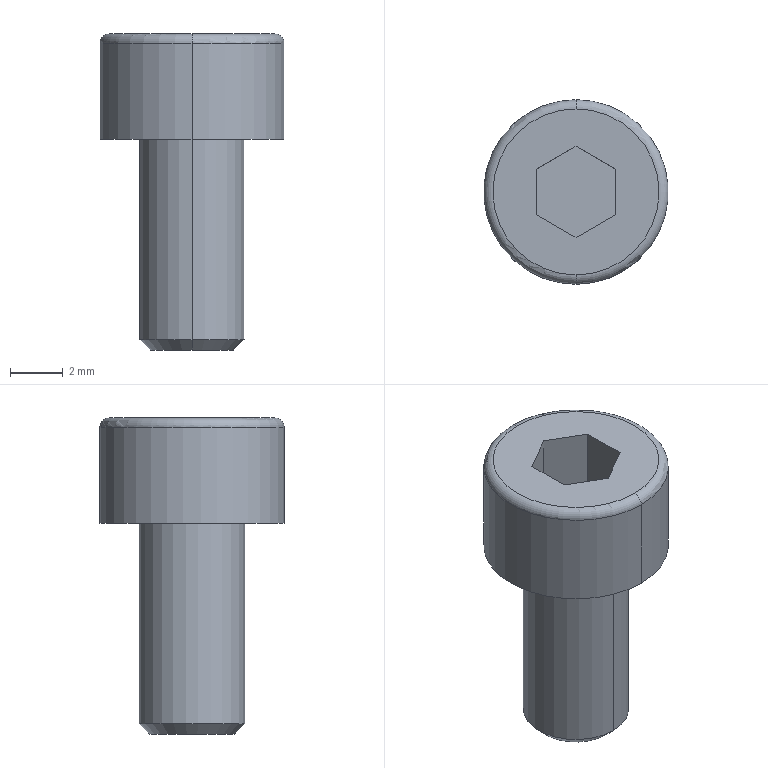Part | SolidWorks | features Chamfer 1, Fillet 1, ICE 1, Revolution 1 | 1 solid | 18 faces | box 7 x 7 x 12 mm | volume 233.87 mm3 | plane 10 | cylinder 4 | cone 2 | torus 2 | commonest cylinder face diameters 4 x2 7 x2
STEP:
#1=CARTESIAN_POINT('',(0.,1.6,-8.));
#2=VERTEX_POINT('',#1);
#3=CARTESIAN_POINT('',(0.,-1.6,-8.));
#4=VERTEX_POINT('',#3);
#5=CARTESIAN_POINT('',(0.,0.,-8.));
#6=DIRECTION('',(0.,0.,-1.));
#7=DIRECTION('',(0.,-1.,0.));
#8=AXIS2_PLACEMENT_3D('',#5,#6,#7);
#9=CIRCLE('',#8,1.6);
#10=EDGE_CURVE('',#2,#4,#9,.T.);
#11=ORIENTED_EDGE('',*,*,#10,.F.);
#12=CARTESIAN_POINT('',(0.,2.,-7.6));
#13=VERTEX_POINT('',#12);
#14=CARTESIAN_POINT('',(0.,2.,-7.6));
#15=DIRECTION('',(0.,0.7071,0.7071));
#16=VECTOR('',#15,1000.);
#17=LINE('',#14,#16);
#18=EDGE_CURVE('',#2,#13,#17,.T.);
#19=ORIENTED_EDGE('',*,*,#18,.T.);
#20=CARTESIAN_POINT('',(0.,-2.,-7.6));
#21=VERTEX_POINT('',#20);
#22=CARTESIAN_POINT('',(0.,0.,-7.6));
#23=DIRECTION('',(0.,0.,1.));
#24=DIRECTION('',(0.,-1.,0.));
#25=AXIS2_PLACEMENT_3D('',#22,#23,#24);
#26=CIRCLE('',#25,2.);
#27=EDGE_CURVE('',#21,#13,#26,.T.);
#28=ORIENTED_EDGE('',*,*,#27,.F.);
#29=CARTESIAN_POINT('',(0.,-2.,-7.6));
#30=DIRECTION('',(0.,-0.7071,0.7071));
#31=VECTOR('',#30,1000.);
#32=LINE('',#29,#31);
#33=EDGE_CURVE('',#4,#21,#32,.T.);
#34=ORIENTED_EDGE('',*,*,#33,.F.);
#35=EDGE_LOOP('',(#11,#19,#28,#34));
#36=FACE_OUTER_BOUND('',#35,.T.);
#37=CARTESIAN_POINT('',(0.,0.,-7.6));
#38=DIRECTION('',(0.,0.,1.));
#39=DIRECTION('',(0.,-1.,0.));
#40=AXIS2_PLACEMENT_3D('',#37,#38,#39);
#41=CONICAL_SURFACE('',#40,2.,0.7854);
#42=ADVANCED_FACE('',(#36),#41,.T.);
#43=CARTESIAN_POINT('',(0.,-3.15,4.));
#44=VERTEX_POINT('',#43);
#45=CARTESIAN_POINT('',(0.,3.15,4.));
#46=VERTEX_POINT('',#45);
#47=CARTESIAN_POINT('',(0.,0.,4.));
#48=DIRECTION('',(0.,0.,1.));
#49=DIRECTION('',(0.,1.,0.));
#50=AXIS2_PLACEMENT_3D('',#47,#48,#49);
#51=CIRCLE('',#50,3.15);
#52=EDGE_CURVE('',#44,#46,#51,.T.);
#53=ORIENTED_EDGE('',*,*,#52,.F.);
#54=CARTESIAN_POINT('',(0.,-3.5,3.65));
#55=VERTEX_POINT('',#54);
#56=CARTESIAN_POINT('',(0.,-3.15,3.65));
#57=DIRECTION('',(1.,0.,0.));
#58=DIRECTION('',(0.,1.,0.));
#59=AXIS2_PLACEMENT_3D('',#56,#57,#58);
#60=CIRCLE('',#59,0.35);
#61=EDGE_CURVE('',#44,#55,#60,.T.);
#62=ORIENTED_EDGE('',*,*,#61,.T.);
#63=CARTESIAN_POINT('',(0.,3.5,3.65));
#64=VERTEX_POINT('',#63);
#65=CARTESIAN_POINT('',(0.,0.,3.65));
#66=DIRECTION('',(0.,0.,-1.));
#67=DIRECTION('',(0.,1.,0.));
#68=AXIS2_PLACEMENT_3D('',#65,#66,#67);
#69=CIRCLE('',#68,3.5);
#70=EDGE_CURVE('',#64,#55,#69,.T.);
#71=ORIENTED_EDGE('',*,*,#70,.F.);
#72=CARTESIAN_POINT('',(0.,3.15,3.65));
#73=DIRECTION('',(-1.,0.,0.));
#74=DIRECTION('',(0.,0.,1.));
#75=AXIS2_PLACEMENT_3D('',#72,#73,#74);
#76=CIRCLE('',#75,0.35);
#77=EDGE_CURVE('',#46,#64,#76,.T.);
#78=ORIENTED_EDGE('',*,*,#77,.F.);
#79=EDGE_LOOP('',(#53,#62,#71,#78));
#80=FACE_OUTER_BOUND('',#79,.T.);
#81=CARTESIAN_POINT('',(0.,0.,3.65));
#82=DIRECTION('',(0.,0.,-1.));
#83=DIRECTION('',(0.,1.,0.));
#84=AXIS2_PLACEMENT_3D('',#81,#82,#83);
#85=TOROIDAL_SURFACE('',#84,3.15,0.35);
#86=ADVANCED_FACE('',(#80),#85,.T.);
#87=ORIENTED_EDGE('',*,*,#27,.T.);
#88=CARTESIAN_POINT('',(0.,2.,0.));
#89=VERTEX_POINT('',#88);
#90=CARTESIAN_POINT('',(0.,2.,4.));
#91=DIRECTION('',(0.,0.,1.));
#92=VECTOR('',#91,1000.);
#93=LINE('',#90,#92);
#94=EDGE_CURVE('',#13,#89,#93,.T.);
#95=ORIENTED_EDGE('',*,*,#94,.T.);
#96=CARTESIAN_POINT('',(0.,-2.,0.));
#97=VERTEX_POINT('',#96);
#98=CARTESIAN_POINT('',(0.,0.,0.));
#99=DIRECTION('',(0.,0.,1.));
#100=DIRECTION('',(0.,-1.,0.));
#101=AXIS2_PLACEMENT_3D('',#98,#99,#100);
#102=CIRCLE('',#101,2.);
#103=EDGE_CURVE('',#97,#89,#102,.T.);
#104=ORIENTED_EDGE('',*,*,#103,.F.);
#105=CARTESIAN_POINT('',(0.,-2.,4.));
#106=DIRECTION('',(0.,0.,1.));
#107=VECTOR('',#106,1000.);
#108=LINE('',#105,#107);
#109=EDGE_CURVE('',#21,#97,#108,.T.);
#110=ORIENTED_EDGE('',*,*,#109,.F.);
#111=EDGE_LOOP('',(#87,#95,#104,#110));
#112=FACE_OUTER_BOUND('',#111,.T.);
#113=CARTESIAN_POINT('',(0.,0.,4.));
#114=DIRECTION('',(0.,0.,1.));
#115=DIRECTION('',(0.,-1.,0.));
#116=AXIS2_PLACEMENT_3D('',#113,#114,#115);
#117=CYLINDRICAL_SURFACE('',#116,2.);
#118=ADVANCED_FACE('',(#112),#117,.T.);
#119=CARTESIAN_POINT('',(0.,-3.5,0.));
#120=VERTEX_POINT('',#119);
#121=CARTESIAN_POINT('',(0.,3.5,0.));
#122=VERTEX_POINT('',#121);
#123=CARTESIAN_POINT('',(0.,0.,0.));
#124=DIRECTION('',(0.,0.,1.));
#125=DIRECTION('',(0.,-1.,0.));
#126=AXIS2_PLACEMENT_3D('',#123,#124,#125);
#127=CIRCLE('',#126,3.5);
#128=EDGE_CURVE('',#120,#122,#127,.T.);
#129=ORIENTED_EDGE('',*,*,#128,.T.);
#130=CARTESIAN_POINT('',(0.,3.5,4.));
#131=DIRECTION('',(0.,0.,1.));
#132=VECTOR('',#131,1000.);
#133=LINE('',#130,#132);
#134=EDGE_CURVE('',#122,#64,#133,.T.);
#135=ORIENTED_EDGE('',*,*,#134,.T.);
#136=ORIENTED_EDGE('',*,*,#70,.T.);
#137=CARTESIAN_POINT('',(0.,-3.5,4.));
#138=DIRECTION('',(0.,0.,1.));
#139=VECTOR('',#138,1000.);
#140=LINE('',#137,#139);
#141=EDGE_CURVE('',#120,#55,#140,.T.);
#142=ORIENTED_EDGE('',*,*,#141,.F.);
#143=EDGE_LOOP('',(#129,#135,#136,#142));
#144=FACE_OUTER_BOUND('',#143,.T.);
#145=CARTESIAN_POINT('',(0.,0.,4.));
#146=DIRECTION('',(0.,0.,1.));
#147=DIRECTION('',(0.,-1.,0.));
#148=AXIS2_PLACEMENT_3D('',#145,#146,#147);
#149=CYLINDRICAL_SURFACE('',#148,3.5);
#150=ADVANCED_FACE('',(#144),#149,.T.);
#151=CARTESIAN_POINT('',(0.,0.,4.));
#152=DIRECTION('',(0.,0.,1.));
#153=DIRECTION('',(0.,1.,0.));
#154=AXIS2_PLACEMENT_3D('',#151,#152,#153);
#155=CIRCLE('',#154,3.15);
#156=EDGE_CURVE('',#46,#44,#155,.T.);
#157=ORIENTED_EDGE('',*,*,#156,.T.);
#158=ORIENTED_EDGE('',*,*,#52,.T.);
#159=EDGE_LOOP('',(#157,#158));
#160=FACE_OUTER_BOUND('',#159,.T.);
#161=CARTESIAN_POINT('',(0.,1.732,4.));
#162=VERTEX_POINT('',#161);
#163=CARTESIAN_POINT('',(-1.5,0.866,4.));
#164=VERTEX_POINT('',#163);
#165=CARTESIAN_POINT('',(0.,1.732,4.));
#166=DIRECTION('',(-0.866,-0.5,0.));
#167=VECTOR('',#166,1000.);
#168=LINE('',#165,#167);
#169=EDGE_CURVE('',#162,#164,#168,.T.);
#170=ORIENTED_EDGE('',*,*,#169,.F.);
#171=CARTESIAN_POINT('',(1.5,0.866,4.));
#172=VERTEX_POINT('',#171);
#173=CARTESIAN_POINT('',(1.5,0.866,4.));
#174=DIRECTION('',(-0.866,0.5,0.));
#175=VECTOR('',#174,1000.);
#176=LINE('',#173,#175);
#177=EDGE_CURVE('',#172,#162,#176,.T.);
#178=ORIENTED_EDGE('',*,*,#177,.F.);
#179=CARTESIAN_POINT('',(1.5,-0.866,4.));
#180=VERTEX_POINT('',#179);
#181=CARTESIAN_POINT('',(1.5,-0.866,4.));
#182=DIRECTION('',(0.,1.,0.));
#183=VECTOR('',#182,1000.);
#184=LINE('',#181,#183);
#185=EDGE_CURVE('',#180,#172,#184,.T.);
#186=ORIENTED_EDGE('',*,*,#185,.F.);
#187=CARTESIAN_POINT('',(0.,-1.732,4.));
#188=VERTEX_POINT('',#187);
#189=CARTESIAN_POINT('',(0.,-1.732,4.));
#190=DIRECTION('',(0.866,0.5,0.));
#191=VECTOR('',#190,1000.);
#192=LINE('',#189,#191);
#193=EDGE_CURVE('',#188,#180,#192,.T.);
#194=ORIENTED_EDGE('',*,*,#193,.F.);
#195=CARTESIAN_POINT('',(-1.5,-0.866,4.));
#196=VERTEX_POINT('',#195);
#197=CARTESIAN_POINT('',(-1.5,-0.866,4.));
#198=DIRECTION('',(0.866,-0.5,0.));
#199=VECTOR('',#198,1000.);
#200=LINE('',#197,#199);
#201=EDGE_CURVE('',#196,#188,#200,.T.);
#202=ORIENTED_EDGE('',*,*,#201,.F.);
#203=CARTESIAN_POINT('',(-1.5,0.866,4.));
#204=DIRECTION('',(0.,-1.,0.));
#205=VECTOR('',#204,1000.);
#206=LINE('',#203,#205);
#207=EDGE_CURVE('',#164,#196,#206,.T.);
#208=ORIENTED_EDGE('',*,*,#207,.F.);
#209=EDGE_LOOP('',(#170,#178,#186,#194,#202,#208));
#210=FACE_BOUND('',#209,.T.);
#211=CARTESIAN_POINT('',(0.,0.,4.));
#212=DIRECTION('',(0.,0.,-1.));
#213=DIRECTION('',(0.,1.,0.));
#214=AXIS2_PLACEMENT_3D('',#211,#212,#213);
#215=PLANE('',#214);
#216=ADVANCED_FACE('',(#160,#210),#215,.F.);
#217=ORIENTED_EDGE('',*,*,#134,.F.);
#218=CARTESIAN_POINT('',(0.,0.,0.));
#219=DIRECTION('',(0.,0.,1.));
#220=DIRECTION('',(0.,-1.,0.));
#221=AXIS2_PLACEMENT_3D('',#218,#219,#220);
#222=CIRCLE('',#221,3.5);
#223=EDGE_CURVE('',#122,#120,#222,.T.);
#224=ORIENTED_EDGE('',*,*,#223,.T.);
#225=ORIENTED_EDGE('',*,*,#141,.T.);
#226=CARTESIAN_POINT('',(0.,0.,3.65));
#227=DIRECTION('',(0.,0.,-1.));
#228=DIRECTION('',(0.,1.,0.));
#229=AXIS2_PLACEMENT_3D('',#226,#227,#228);
#230=CIRCLE('',#229,3.5);
#231=EDGE_CURVE('',#55,#64,#230,.T.);
#232=ORIENTED_EDGE('',*,*,#231,.T.);
#233=EDGE_LOOP('',(#217,#224,#225,#232));
#234=FACE_OUTER_BOUND('',#233,.T.);
#235=CARTESIAN_POINT('',(0.,0.,4.));
#236=DIRECTION('',(0.,0.,1.));
#237=DIRECTION('',(0.,-1.,0.));
#238=AXIS2_PLACEMENT_3D('',#235,#236,#237);
#239=CYLINDRICAL_SURFACE('',#238,3.5);
#240=ADVANCED_FACE('',(#234),#239,.T.);
#241=ORIENTED_EDGE('',*,*,#128,.F.);
#242=ORIENTED_EDGE('',*,*,#223,.F.);
#243=EDGE_LOOP('',(#241,#242));
#244=FACE_OUTER_BOUND('',#243,.T.);
#245=ORIENTED_EDGE('',*,*,#103,.T.);
#246=CARTESIAN_POINT('',(0.,0.,0.));
#247=DIRECTION('',(0.,0.,1.));
#248=DIRECTION('',(0.,-1.,0.));
#249=AXIS2_PLACEMENT_3D('',#246,#247,#248);
#250=CIRCLE('',#249,2.);
#251=EDGE_CURVE('',#89,#97,#250,.T.);
#252=ORIENTED_EDGE('',*,*,#251,.T.);
#253=EDGE_LOOP('',(#245,#252));
#254=FACE_BOUND('',#253,.T.);
#255=CARTESIAN_POINT('',(0.,3.5,0.));
#256=DIRECTION('',(0.,0.,1.));
#257=DIRECTION('',(0.,-1.,0.));
#258=AXIS2_PLACEMENT_3D('',#255,#256,#257);
#259=PLANE('',#258);
#260=ADVANCED_FACE('',(#244,#254),#259,.F.);
#261=ORIENTED_EDGE('',*,*,#94,.F.);
#262=CARTESIAN_POINT('',(0.,0.,-7.6));
#263=DIRECTION('',(0.,0.,1.));
#264=DIRECTION('',(0.,-1.,0.));
#265=AXIS2_PLACEMENT_3D('',#262,#263,#264);
#266=CIRCLE('',#265,2.);
#267=EDGE_CURVE('',#13,#21,#266,.T.);
#268=ORIENTED_EDGE('',*,*,#267,.T.);
#269=ORIENTED_EDGE('',*,*,#109,.T.);
#270=ORIENTED_EDGE('',*,*,#251,.F.);
#271=EDGE_LOOP('',(#261,#268,#269,#270));
#272=FACE_OUTER_BOUND('',#271,.T.);
#273=CARTESIAN_POINT('',(0.,0.,4.));
#274=DIRECTION('',(0.,0.,1.));
#275=DIRECTION('',(0.,-1.,0.));
#276=AXIS2_PLACEMENT_3D('',#273,#274,#275);
#277=CYLINDRICAL_SURFACE('',#276,2.);
#278=ADVANCED_FACE('',(#272),#277,.T.);
#279=CARTESIAN_POINT('',(0.,0.,-8.));
#280=DIRECTION('',(0.,0.,-1.));
#281=DIRECTION('',(0.,-1.,0.));
#282=AXIS2_PLACEMENT_3D('',#279,#280,#281);
#283=CIRCLE('',#282,1.6);
#284=EDGE_CURVE('',#4,#2,#283,.T.);
#285=ORIENTED_EDGE('',*,*,#284,.T.);
#286=ORIENTED_EDGE('',*,*,#10,.T.);
#287=EDGE_LOOP('',(#285,#286));
#288=FACE_OUTER_BOUND('',#287,.T.);
#289=CARTESIAN_POINT('',(0.,2.,-8.));
#290=DIRECTION('',(0.,0.,1.));
#291=DIRECTION('',(0.,-1.,0.));
#292=AXIS2_PLACEMENT_3D('',#289,#290,#291);
#293=PLANE('',#292);
#294=ADVANCED_FACE('',(#288),#293,.F.);
#295=ORIENTED_EDGE('',*,*,#177,.T.);
#296=CARTESIAN_POINT('',(0.,1.732,1.55));
#297=VERTEX_POINT('',#296);
#298=CARTESIAN_POINT('',(0.,1.732,1.55));
#299=DIRECTION('',(0.,0.,1.));
#300=VECTOR('',#299,1000.);
#301=LINE('',#298,#300);
#302=EDGE_CURVE('',#297,#162,#301,.T.);
#303=ORIENTED_EDGE('',*,*,#302,.F.);
#304=CARTESIAN_POINT('',(1.5,0.866,1.55));
#305=VERTEX_POINT('',#304);
#306=CARTESIAN_POINT('',(1.5,0.866,1.55));
#307=DIRECTION('',(-0.866,0.5,0.));
#308=VECTOR('',#307,1000.);
#309=LINE('',#306,#308);
#310=EDGE_CURVE('',#305,#297,#309,.T.);
#311=ORIENTED_EDGE('',*,*,#310,.F.);
#312=CARTESIAN_POINT('',(1.5,0.866,1.55));
#313=DIRECTION('',(0.,0.,1.));
#314=VECTOR('',#313,1000.);
#315=LINE('',#312,#314);
#316=EDGE_CURVE('',#305,#172,#315,.T.);
#317=ORIENTED_EDGE('',*,*,#316,.T.);
#318=EDGE_LOOP('',(#295,#303,#311,#317));
#319=FACE_OUTER_BOUND('',#318,.T.);
#320=CARTESIAN_POINT('',(1.5,0.866,1.55));
#321=DIRECTION('',(0.5,0.866,0.));
#322=DIRECTION('',(-0.866,0.5,0.));
#323=AXIS2_PLACEMENT_3D('',#320,#321,#322);
#324=PLANE('',#323);
#325=ADVANCED_FACE('',(#319),#324,.F.);
#326=ORIENTED_EDGE('',*,*,#185,.T.);
#327=ORIENTED_EDGE('',*,*,#316,.F.);
#328=CARTESIAN_POINT('',(1.5,-0.866,1.55));
#329=VERTEX_POINT('',#328);
#330=CARTESIAN_POINT('',(1.5,-0.866,1.55));
#331=DIRECTION('',(0.,1.,0.));
#332=VECTOR('',#331,1000.);
#333=LINE('',#330,#332);
#334=EDGE_CURVE('',#329,#305,#333,.T.);
#335=ORIENTED_EDGE('',*,*,#334,.F.);
#336=CARTESIAN_POINT('',(1.5,-0.866,1.55));
#337=DIRECTION('',(0.,0.,1.));
#338=VECTOR('',#337,1000.);
#339=LINE('',#336,#338);
#340=EDGE_CURVE('',#329,#180,#339,.T.);
#341=ORIENTED_EDGE('',*,*,#340,.T.);
#342=EDGE_LOOP('',(#326,#327,#335,#341));
#343=FACE_OUTER_BOUND('',#342,.T.);
#344=CARTESIAN_POINT('',(1.5,-0.866,1.55));
#345=DIRECTION('',(1.,0.,0.));
#346=DIRECTION('',(0.,0.,-1.));
#347=AXIS2_PLACEMENT_3D('',#344,#345,#346);
#348=PLANE('',#347);
#349=ADVANCED_FACE('',(#343),#348,.F.);
#350=ORIENTED_EDGE('',*,*,#193,.T.);
#351=ORIENTED_EDGE('',*,*,#340,.F.);
#352=CARTESIAN_POINT('',(0.,-1.732,1.55));
#353=VERTEX_POINT('',#352);
#354=CARTESIAN_POINT('',(0.,-1.732,1.55));
#355=DIRECTION('',(0.866,0.5,0.));
#356=VECTOR('',#355,1000.);
#357=LINE('',#354,#356);
#358=EDGE_CURVE('',#353,#329,#357,.T.);
#359=ORIENTED_EDGE('',*,*,#358,.F.);
#360=CARTESIAN_POINT('',(0.,-1.732,1.55));
#361=DIRECTION('',(0.,0.,1.));
#362=VECTOR('',#361,1000.);
#363=LINE('',#360,#362);
#364=EDGE_CURVE('',#353,#188,#363,.T.);
#365=ORIENTED_EDGE('',*,*,#364,.T.);
#366=EDGE_LOOP('',(#350,#351,#359,#365));
#367=FACE_OUTER_BOUND('',#366,.T.);
#368=CARTESIAN_POINT('',(0.,-1.732,1.55));
#369=DIRECTION('',(0.5,-0.866,0.));
#370=DIRECTION('',(0.866,0.5,0.));
#371=AXIS2_PLACEMENT_3D('',#368,#369,#370);
#372=PLANE('',#371);
#373=ADVANCED_FACE('',(#367),#372,.F.);
#374=ORIENTED_EDGE('',*,*,#201,.T.);
#375=ORIENTED_EDGE('',*,*,#364,.F.);
#376=CARTESIAN_POINT('',(-1.5,-0.866,1.55));
#377=VERTEX_POINT('',#376);
#378=CARTESIAN_POINT('',(-1.5,-0.866,1.55));
#379=DIRECTION('',(0.866,-0.5,0.));
#380=VECTOR('',#379,1000.);
#381=LINE('',#378,#380);
#382=EDGE_CURVE('',#377,#353,#381,.T.);
#383=ORIENTED_EDGE('',*,*,#382,.F.);
#384=CARTESIAN_POINT('',(-1.5,-0.866,1.55));
#385=DIRECTION('',(0.,0.,1.));
#386=VECTOR('',#385,1000.);
#387=LINE('',#384,#386);
#388=EDGE_CURVE('',#377,#196,#387,.T.);
#389=ORIENTED_EDGE('',*,*,#388,.T.);
#390=EDGE_LOOP('',(#374,#375,#383,#389));
#391=FACE_OUTER_BOUND('',#390,.T.);
#392=CARTESIAN_POINT('',(-1.5,-0.866,1.55));
#393=DIRECTION('',(-0.5,-0.866,0.));
#394=DIRECTION('',(0.866,-0.5,0.));
#395=AXIS2_PLACEMENT_3D('',#392,#393,#394);
#396=PLANE('',#395);
#397=ADVANCED_FACE('',(#391),#396,.F.);
#398=ORIENTED_EDGE('',*,*,#207,.T.);
#399=ORIENTED_EDGE('',*,*,#388,.F.);
#400=CARTESIAN_POINT('',(-1.5,0.866,1.55));
#401=VERTEX_POINT('',#400);
#402=CARTESIAN_POINT('',(-1.5,0.866,1.55));
#403=DIRECTION('',(0.,-1.,0.));
#404=VECTOR('',#403,1000.);
#405=LINE('',#402,#404);
#406=EDGE_CURVE('',#401,#377,#405,.T.);
#407=ORIENTED_EDGE('',*,*,#406,.F.);
#408=CARTESIAN_POINT('',(-1.5,0.866,1.55));
#409=DIRECTION('',(0.,0.,1.));
#410=VECTOR('',#409,1000.);
#411=LINE('',#408,#410);
#412=EDGE_CURVE('',#401,#164,#411,.T.);
#413=ORIENTED_EDGE('',*,*,#412,.T.);
#414=EDGE_LOOP('',(#398,#399,#407,#413));
#415=FACE_OUTER_BOUND('',#414,.T.);
#416=CARTESIAN_POINT('',(-1.5,0.866,1.55));
#417=DIRECTION('',(-1.,0.,0.));
#418=DIRECTION('',(0.,0.,1.));
#419=AXIS2_PLACEMENT_3D('',#416,#417,#418);
#420=PLANE('',#419);
#421=ADVANCED_FACE('',(#415),#420,.F.);
#422=ORIENTED_EDGE('',*,*,#169,.T.);
#423=ORIENTED_EDGE('',*,*,#412,.F.);
#424=CARTESIAN_POINT('',(0.,1.732,1.55));
#425=DIRECTION('',(-0.866,-0.5,0.));
#426=VECTOR('',#425,1000.);
#427=LINE('',#424,#426);
#428=EDGE_CURVE('',#297,#401,#427,.T.);
#429=ORIENTED_EDGE('',*,*,#428,.F.);
#430=ORIENTED_EDGE('',*,*,#302,.T.);
#431=EDGE_LOOP('',(#422,#423,#429,#430));
#432=FACE_OUTER_BOUND('',#431,.T.);
#433=CARTESIAN_POINT('',(0.,1.732,1.55));
#434=DIRECTION('',(-0.5,0.866,0.));
#435=DIRECTION('',(-0.866,-0.5,0.));
#436=AXIS2_PLACEMENT_3D('',#433,#434,#435);
#437=PLANE('',#436);
#438=ADVANCED_FACE('',(#432),#437,.F.);
#439=ORIENTED_EDGE('',*,*,#310,.T.);
#440=ORIENTED_EDGE('',*,*,#428,.T.);
#441=ORIENTED_EDGE('',*,*,#406,.T.);
#442=ORIENTED_EDGE('',*,*,#382,.T.);
#443=ORIENTED_EDGE('',*,*,#358,.T.);
#444=ORIENTED_EDGE('',*,*,#334,.T.);
#445=EDGE_LOOP('',(#439,#440,#441,#442,#443,#444));
#446=FACE_OUTER_BOUND('',#445,.T.);
#447=CARTESIAN_POINT('',(0.,1.732,1.55));
#448=DIRECTION('',(0.,0.,1.));
#449=DIRECTION('',(1.,0.,0.));
#450=AXIS2_PLACEMENT_3D('',#447,#448,#449);
#451=PLANE('',#450);
#452=ADVANCED_FACE('',(#446),#451,.T.);
#453=ORIENTED_EDGE('',*,*,#61,.F.);
#454=ORIENTED_EDGE('',*,*,#156,.F.);
#455=ORIENTED_EDGE('',*,*,#77,.T.);
#456=ORIENTED_EDGE('',*,*,#231,.F.);
#457=EDGE_LOOP('',(#453,#454,#455,#456));
#458=FACE_OUTER_BOUND('',#457,.T.);
#459=CARTESIAN_POINT('',(0.,0.,3.65));
#460=DIRECTION('',(0.,0.,-1.));
#461=DIRECTION('',(0.,1.,0.));
#462=AXIS2_PLACEMENT_3D('',#459,#460,#461);
#463=TOROIDAL_SURFACE('',#462,3.15,0.35);
#464=ADVANCED_FACE('',(#458),#463,.T.);
#465=ORIENTED_EDGE('',*,*,#18,.F.);
#466=ORIENTED_EDGE('',*,*,#284,.F.);
#467=ORIENTED_EDGE('',*,*,#33,.T.);
#468=ORIENTED_EDGE('',*,*,#267,.F.);
#469=EDGE_LOOP('',(#465,#466,#467,#468));
#470=FACE_OUTER_BOUND('',#469,.T.);
#471=CARTESIAN_POINT('',(0.,0.,-7.6));
#472=DIRECTION('',(0.,0.,1.));
#473=DIRECTION('',(0.,-1.,0.));
#474=AXIS2_PLACEMENT_3D('',#471,#472,#473);
#475=CONICAL_SURFACE('',#474,2.,0.7854);
#476=ADVANCED_FACE('',(#470),#475,.T.);
#477=CLOSED_SHELL('',(#42,#86,#118,#150,#216,#240,#260,#278,#294,#325,#349,#373,#397,#421,#438,#452,#464,#476));
#478=MANIFOLD_SOLID_BREP('',#477);
#479=CARTESIAN_POINT('',(0.,0.,0.));
#480=DIRECTION('',(0.,0.,1.));
#481=DIRECTION('',(1.,0.,0.));
#482=AXIS2_PLACEMENT_3D('',#479,#480,#481);
#483=(LENGTH_UNIT()NAMED_UNIT(*)SI_UNIT(.MILLI.,.METRE.));
#484=UNCERTAINTY_MEASURE_WITH_UNIT(LENGTH_MEASURE(0.00001),#483,'','');
#485=(NAMED_UNIT(*)PLANE_ANGLE_UNIT()SI_UNIT($,.RADIAN.));
#486=(NAMED_UNIT(*)SI_UNIT($,.STERADIAN.)SOLID_ANGLE_UNIT());
#487=(GEOMETRIC_REPRESENTATION_CONTEXT(3)GLOBAL_UNCERTAINTY_ASSIGNED_CONTEXT((#484))GLOBAL_UNIT_ASSIGNED_CONTEXT((#483,#485,#486))REPRESENTATION_CONTEXT('',''));
#488=ADVANCED_BREP_SHAPE_REPRESENTATION('',(#478,#482),#487);